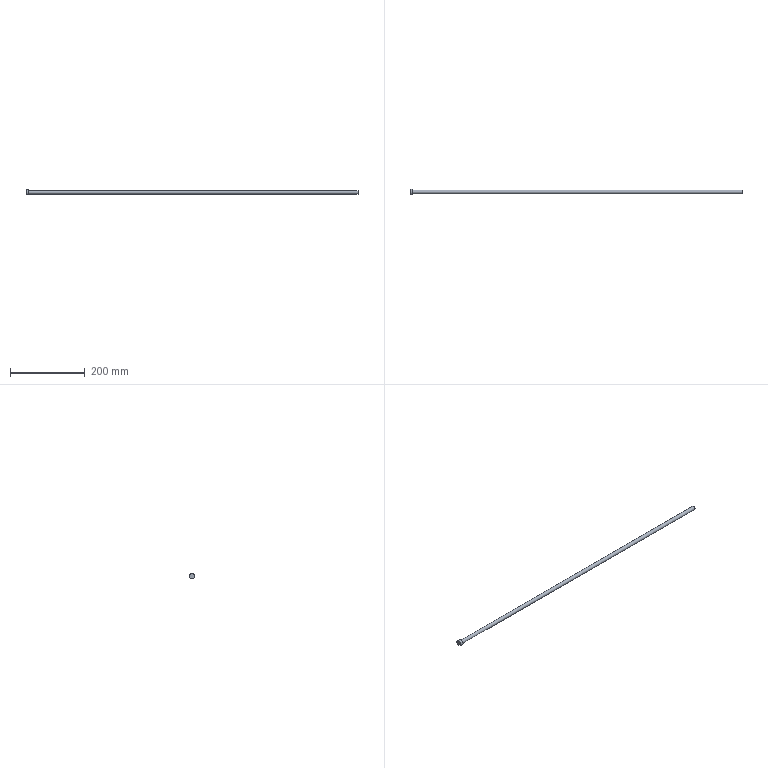Part | STEP file | solid 38 | 1 solid | 6 faces | box 890 x 15 x 13 mm | volume 70574 mm3 | plane 4 | cylinder 2 | commonest cylinder face diameters 10 x1 15 x1